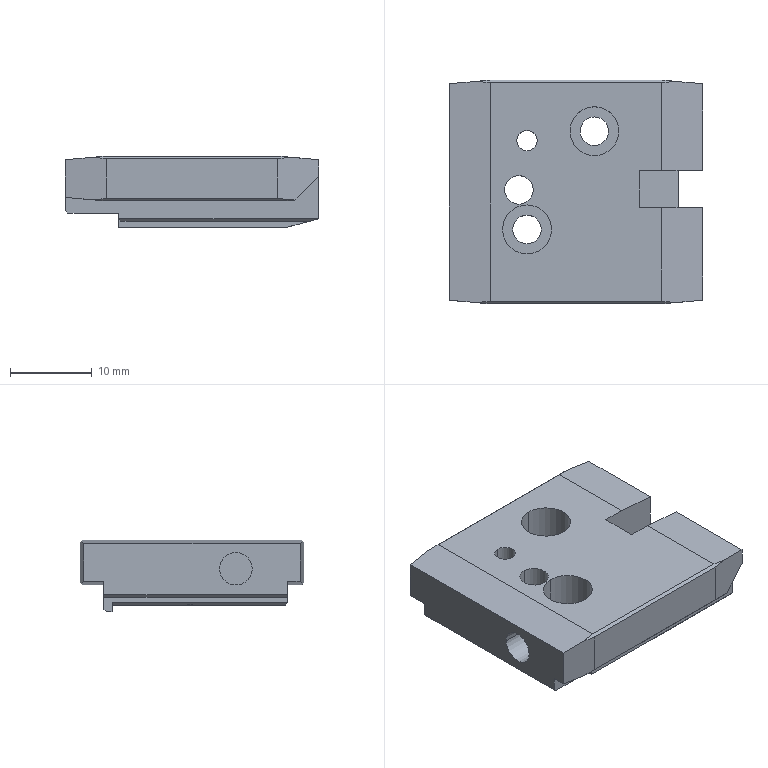Part | NX | 1 solid | 67 faces | box 31 x 27.4 x 8.8 mm | volume 5502 mm3 | plane 51 | cylinder 16 | commonest cylinder face diameters 3.5 x6 6 x4 1 x2 2.5 x2 4 x2